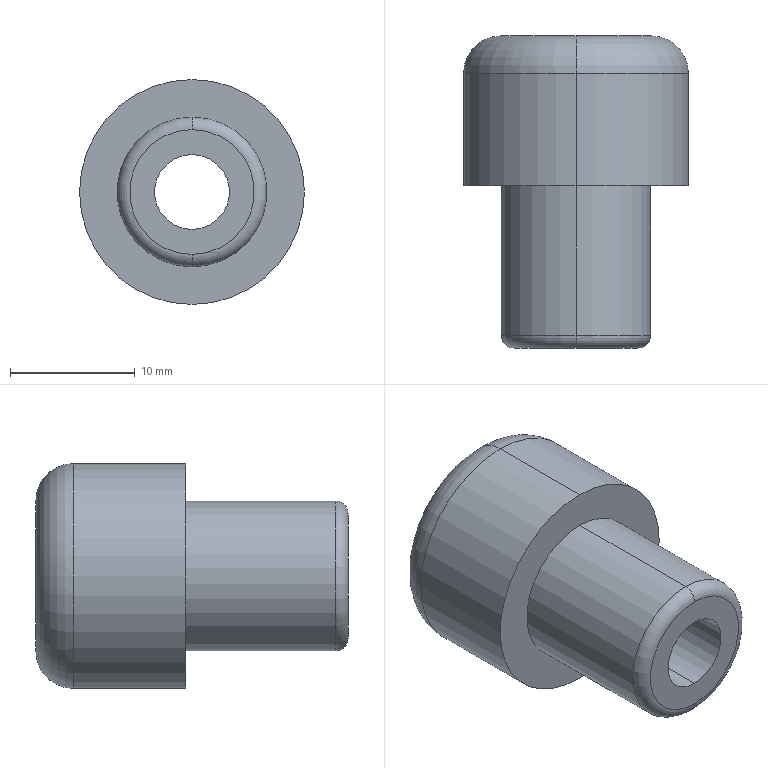Part | SolidWorks | features Fillet 2, Revolution 1 | 1 solid | 13 faces | box 18 x 25 x 18 mm | volume 3708 mm3 | cylinder 6 | torus 4 | plane 3 | commonest cylinder face diameters 6 x2 12 x2 18 x2
STEP:
#1=CARTESIAN_POINT('',(0.,1.,6.));
#2=VERTEX_POINT('',#1);
#3=CARTESIAN_POINT('',(0.,1.,-6.));
#4=VERTEX_POINT('',#3);
#5=CARTESIAN_POINT('',(0.,1.,0.));
#6=DIRECTION('',(0.,1.,0.));
#7=DIRECTION('',(0.,0.,-1.));
#8=AXIS2_PLACEMENT_3D('',#5,#6,#7);
#9=CIRCLE('',#8,6.);
#10=EDGE_CURVE('',#2,#4,#9,.T.);
#11=ORIENTED_EDGE('',*,*,#10,.F.);
#12=CARTESIAN_POINT('',(0.,0.,5.));
#13=VERTEX_POINT('',#12);
#14=CARTESIAN_POINT('',(0.,1.,5.));
#15=DIRECTION('',(1.,0.,0.));
#16=DIRECTION('',(0.,0.,-1.));
#17=AXIS2_PLACEMENT_3D('',#14,#15,#16);
#18=CIRCLE('',#17,1.);
#19=EDGE_CURVE('',#2,#13,#18,.T.);
#20=ORIENTED_EDGE('',*,*,#19,.T.);
#21=CARTESIAN_POINT('',(0.,0.,-5.));
#22=VERTEX_POINT('',#21);
#23=CARTESIAN_POINT('',(0.,0.,0.));
#24=DIRECTION('',(0.,-1.,0.));
#25=DIRECTION('',(0.,0.,-1.));
#26=AXIS2_PLACEMENT_3D('',#23,#24,#25);
#27=CIRCLE('',#26,5.);
#28=EDGE_CURVE('',#22,#13,#27,.T.);
#29=ORIENTED_EDGE('',*,*,#28,.F.);
#30=CARTESIAN_POINT('',(0.,1.,-5.));
#31=DIRECTION('',(-1.,0.,0.));
#32=DIRECTION('',(0.,0.,1.));
#33=AXIS2_PLACEMENT_3D('',#30,#31,#32);
#34=CIRCLE('',#33,1.);
#35=EDGE_CURVE('',#4,#22,#34,.T.);
#36=ORIENTED_EDGE('',*,*,#35,.F.);
#37=EDGE_LOOP('',(#11,#20,#29,#36));
#38=FACE_OUTER_BOUND('',#37,.T.);
#39=CARTESIAN_POINT('',(0.,1.,0.));
#40=DIRECTION('',(0.,-1.,0.));
#41=DIRECTION('',(0.,0.,-1.));
#42=AXIS2_PLACEMENT_3D('',#39,#40,#41);
#43=TOROIDAL_SURFACE('',#42,5.,1.);
#44=ADVANCED_FACE('',(#38),#43,.T.);
#45=CARTESIAN_POINT('',(0.,22.,-9.));
#46=VERTEX_POINT('',#45);
#47=CARTESIAN_POINT('',(0.,22.,9.));
#48=VERTEX_POINT('',#47);
#49=CARTESIAN_POINT('',(0.,22.,0.));
#50=DIRECTION('',(0.,-1.,0.));
#51=DIRECTION('',(0.,0.,1.));
#52=AXIS2_PLACEMENT_3D('',#49,#50,#51);
#53=CIRCLE('',#52,9.);
#54=EDGE_CURVE('',#46,#48,#53,.T.);
#55=ORIENTED_EDGE('',*,*,#54,.F.);
#56=CARTESIAN_POINT('',(0.,25.,-6.));
#57=VERTEX_POINT('',#56);
#58=CARTESIAN_POINT('',(0.,22.,-6.));
#59=DIRECTION('',(1.,0.,0.));
#60=DIRECTION('',(0.,0.,-1.));
#61=AXIS2_PLACEMENT_3D('',#58,#59,#60);
#62=CIRCLE('',#61,3.);
#63=EDGE_CURVE('',#46,#57,#62,.T.);
#64=ORIENTED_EDGE('',*,*,#63,.T.);
#65=CARTESIAN_POINT('',(0.,25.,6.));
#66=VERTEX_POINT('',#65);
#67=CARTESIAN_POINT('',(0.,25.,0.));
#68=DIRECTION('',(0.,1.,0.));
#69=DIRECTION('',(0.,0.,1.));
#70=AXIS2_PLACEMENT_3D('',#67,#68,#69);
#71=CIRCLE('',#70,6.);
#72=EDGE_CURVE('',#66,#57,#71,.T.);
#73=ORIENTED_EDGE('',*,*,#72,.F.);
#74=CARTESIAN_POINT('',(0.,22.,6.));
#75=DIRECTION('',(-1.,0.,0.));
#76=DIRECTION('',(0.,0.,1.));
#77=AXIS2_PLACEMENT_3D('',#74,#75,#76);
#78=CIRCLE('',#77,3.);
#79=EDGE_CURVE('',#48,#66,#78,.T.);
#80=ORIENTED_EDGE('',*,*,#79,.F.);
#81=EDGE_LOOP('',(#55,#64,#73,#80));
#82=FACE_OUTER_BOUND('',#81,.T.);
#83=CARTESIAN_POINT('',(0.,22.,0.));
#84=DIRECTION('',(0.,1.,0.));
#85=DIRECTION('',(0.,0.,1.));
#86=AXIS2_PLACEMENT_3D('',#83,#84,#85);
#87=TOROIDAL_SURFACE('',#86,6.,3.);
#88=ADVANCED_FACE('',(#82),#87,.T.);
#89=ORIENTED_EDGE('',*,*,#54,.T.);
#90=CARTESIAN_POINT('',(0.,13.,9.));
#91=VERTEX_POINT('',#90);
#92=CARTESIAN_POINT('',(0.,0.,9.));
#93=DIRECTION('',(0.,-1.,0.));
#94=VECTOR('',#93,1000.);
#95=LINE('',#92,#94);
#96=EDGE_CURVE('',#48,#91,#95,.T.);
#97=ORIENTED_EDGE('',*,*,#96,.T.);
#98=CARTESIAN_POINT('',(0.,13.,-9.));
#99=VERTEX_POINT('',#98);
#100=CARTESIAN_POINT('',(0.,13.,0.));
#101=DIRECTION('',(0.,-1.,0.));
#102=DIRECTION('',(0.,0.,-1.));
#103=AXIS2_PLACEMENT_3D('',#100,#101,#102);
#104=CIRCLE('',#103,9.);
#105=EDGE_CURVE('',#99,#91,#104,.T.);
#106=ORIENTED_EDGE('',*,*,#105,.F.);
#107=CARTESIAN_POINT('',(0.,0.,-9.));
#108=DIRECTION('',(0.,-1.,0.));
#109=VECTOR('',#108,1000.);
#110=LINE('',#107,#109);
#111=EDGE_CURVE('',#46,#99,#110,.T.);
#112=ORIENTED_EDGE('',*,*,#111,.F.);
#113=EDGE_LOOP('',(#89,#97,#106,#112));
#114=FACE_OUTER_BOUND('',#113,.T.);
#115=CARTESIAN_POINT('',(0.,0.,0.));
#116=DIRECTION('',(0.,-1.,0.));
#117=DIRECTION('',(0.,0.,-1.));
#118=AXIS2_PLACEMENT_3D('',#115,#116,#117);
#119=CYLINDRICAL_SURFACE('',#118,9.);
#120=ADVANCED_FACE('',(#114),#119,.T.);
#121=CARTESIAN_POINT('',(0.,13.,-6.));
#122=VERTEX_POINT('',#121);
#123=CARTESIAN_POINT('',(0.,13.,6.));
#124=VERTEX_POINT('',#123);
#125=CARTESIAN_POINT('',(0.,13.,0.));
#126=DIRECTION('',(0.,-1.,0.));
#127=DIRECTION('',(0.,0.,-1.));
#128=AXIS2_PLACEMENT_3D('',#125,#126,#127);
#129=CIRCLE('',#128,6.);
#130=EDGE_CURVE('',#122,#124,#129,.T.);
#131=ORIENTED_EDGE('',*,*,#130,.T.);
#132=CARTESIAN_POINT('',(0.,0.,6.));
#133=DIRECTION('',(0.,-1.,0.));
#134=VECTOR('',#133,1000.);
#135=LINE('',#132,#134);
#136=EDGE_CURVE('',#124,#2,#135,.T.);
#137=ORIENTED_EDGE('',*,*,#136,.T.);
#138=ORIENTED_EDGE('',*,*,#10,.T.);
#139=CARTESIAN_POINT('',(0.,0.,-6.));
#140=DIRECTION('',(0.,-1.,0.));
#141=VECTOR('',#140,1000.);
#142=LINE('',#139,#141);
#143=EDGE_CURVE('',#122,#4,#142,.T.);
#144=ORIENTED_EDGE('',*,*,#143,.F.);
#145=EDGE_LOOP('',(#131,#137,#138,#144));
#146=FACE_OUTER_BOUND('',#145,.T.);
#147=CARTESIAN_POINT('',(0.,0.,0.));
#148=DIRECTION('',(0.,-1.,0.));
#149=DIRECTION('',(0.,0.,-1.));
#150=AXIS2_PLACEMENT_3D('',#147,#148,#149);
#151=CYLINDRICAL_SURFACE('',#150,6.);
#152=ADVANCED_FACE('',(#146),#151,.T.);
#153=CARTESIAN_POINT('',(0.,25.,3.));
#154=VERTEX_POINT('',#153);
#155=CARTESIAN_POINT('',(0.,25.,-3.));
#156=VERTEX_POINT('',#155);
#157=CARTESIAN_POINT('',(0.,25.,0.));
#158=DIRECTION('',(0.,-1.,0.));
#159=DIRECTION('',(0.,0.,-1.));
#160=AXIS2_PLACEMENT_3D('',#157,#158,#159);
#161=CIRCLE('',#160,3.);
#162=EDGE_CURVE('',#154,#156,#161,.T.);
#163=ORIENTED_EDGE('',*,*,#162,.F.);
#164=CARTESIAN_POINT('',(0.,0.,3.));
#165=VERTEX_POINT('',#164);
#166=CARTESIAN_POINT('',(0.,0.,3.));
#167=DIRECTION('',(0.,-1.,0.));
#168=VECTOR('',#167,1000.);
#169=LINE('',#166,#168);
#170=EDGE_CURVE('',#154,#165,#169,.T.);
#171=ORIENTED_EDGE('',*,*,#170,.T.);
#172=CARTESIAN_POINT('',(0.,0.,-3.));
#173=VERTEX_POINT('',#172);
#174=CARTESIAN_POINT('',(0.,0.,0.));
#175=DIRECTION('',(0.,-1.,0.));
#176=DIRECTION('',(0.,0.,-1.));
#177=AXIS2_PLACEMENT_3D('',#174,#175,#176);
#178=CIRCLE('',#177,3.);
#179=EDGE_CURVE('',#165,#173,#178,.T.);
#180=ORIENTED_EDGE('',*,*,#179,.T.);
#181=CARTESIAN_POINT('',(0.,0.,-3.));
#182=DIRECTION('',(0.,-1.,0.));
#183=VECTOR('',#182,1000.);
#184=LINE('',#181,#183);
#185=EDGE_CURVE('',#156,#173,#184,.T.);
#186=ORIENTED_EDGE('',*,*,#185,.F.);
#187=EDGE_LOOP('',(#163,#171,#180,#186));
#188=FACE_OUTER_BOUND('',#187,.T.);
#189=CARTESIAN_POINT('',(0.,0.,0.));
#190=DIRECTION('',(0.,-1.,0.));
#191=DIRECTION('',(0.,0.,-1.));
#192=AXIS2_PLACEMENT_3D('',#189,#190,#191);
#193=CYLINDRICAL_SURFACE('',#192,3.);
#194=ADVANCED_FACE('',(#188),#193,.F.);
#195=ORIENTED_EDGE('',*,*,#72,.T.);
#196=CARTESIAN_POINT('',(0.,25.,0.));
#197=DIRECTION('',(0.,1.,0.));
#198=DIRECTION('',(0.,0.,1.));
#199=AXIS2_PLACEMENT_3D('',#196,#197,#198);
#200=CIRCLE('',#199,6.);
#201=EDGE_CURVE('',#57,#66,#200,.T.);
#202=ORIENTED_EDGE('',*,*,#201,.T.);
#203=EDGE_LOOP('',(#195,#202));
#204=FACE_OUTER_BOUND('',#203,.T.);
#205=CARTESIAN_POINT('',(0.,25.,0.));
#206=DIRECTION('',(0.,-1.,0.));
#207=DIRECTION('',(0.,0.,-1.));
#208=AXIS2_PLACEMENT_3D('',#205,#206,#207);
#209=CIRCLE('',#208,3.);
#210=EDGE_CURVE('',#156,#154,#209,.T.);
#211=ORIENTED_EDGE('',*,*,#210,.T.);
#212=ORIENTED_EDGE('',*,*,#162,.T.);
#213=EDGE_LOOP('',(#211,#212));
#214=FACE_BOUND('',#213,.T.);
#215=CARTESIAN_POINT('',(9.,25.,0.));
#216=DIRECTION('',(0.,1.,0.));
#217=DIRECTION('',(0.,0.,1.));
#218=AXIS2_PLACEMENT_3D('',#215,#216,#217);
#219=PLANE('',#218);
#220=ADVANCED_FACE('',(#204,#214),#219,.T.);
#221=ORIENTED_EDGE('',*,*,#170,.F.);
#222=ORIENTED_EDGE('',*,*,#210,.F.);
#223=ORIENTED_EDGE('',*,*,#185,.T.);
#224=CARTESIAN_POINT('',(0.,0.,0.));
#225=DIRECTION('',(0.,-1.,0.));
#226=DIRECTION('',(0.,0.,-1.));
#227=AXIS2_PLACEMENT_3D('',#224,#225,#226);
#228=CIRCLE('',#227,3.);
#229=EDGE_CURVE('',#173,#165,#228,.T.);
#230=ORIENTED_EDGE('',*,*,#229,.T.);
#231=EDGE_LOOP('',(#221,#222,#223,#230));
#232=FACE_OUTER_BOUND('',#231,.T.);
#233=CARTESIAN_POINT('',(0.,0.,0.));
#234=DIRECTION('',(0.,-1.,0.));
#235=DIRECTION('',(0.,0.,-1.));
#236=AXIS2_PLACEMENT_3D('',#233,#234,#235);
#237=CYLINDRICAL_SURFACE('',#236,3.);
#238=ADVANCED_FACE('',(#232),#237,.F.);
#239=ORIENTED_EDGE('',*,*,#28,.T.);
#240=CARTESIAN_POINT('',(0.,0.,0.));
#241=DIRECTION('',(0.,-1.,0.));
#242=DIRECTION('',(0.,0.,-1.));
#243=AXIS2_PLACEMENT_3D('',#240,#241,#242);
#244=CIRCLE('',#243,5.);
#245=EDGE_CURVE('',#13,#22,#244,.T.);
#246=ORIENTED_EDGE('',*,*,#245,.T.);
#247=EDGE_LOOP('',(#239,#246));
#248=FACE_OUTER_BOUND('',#247,.T.);
#249=ORIENTED_EDGE('',*,*,#229,.F.);
#250=ORIENTED_EDGE('',*,*,#179,.F.);
#251=EDGE_LOOP('',(#249,#250));
#252=FACE_BOUND('',#251,.T.);
#253=CARTESIAN_POINT('',(3.,0.,0.));
#254=DIRECTION('',(0.,-1.,0.));
#255=DIRECTION('',(0.,0.,-1.));
#256=AXIS2_PLACEMENT_3D('',#253,#254,#255);
#257=PLANE('',#256);
#258=ADVANCED_FACE('',(#248,#252),#257,.T.);
#259=ORIENTED_EDGE('',*,*,#136,.F.);
#260=CARTESIAN_POINT('',(0.,13.,0.));
#261=DIRECTION('',(0.,-1.,0.));
#262=DIRECTION('',(0.,0.,-1.));
#263=AXIS2_PLACEMENT_3D('',#260,#261,#262);
#264=CIRCLE('',#263,6.);
#265=EDGE_CURVE('',#124,#122,#264,.T.);
#266=ORIENTED_EDGE('',*,*,#265,.T.);
#267=ORIENTED_EDGE('',*,*,#143,.T.);
#268=CARTESIAN_POINT('',(0.,1.,0.));
#269=DIRECTION('',(0.,1.,0.));
#270=DIRECTION('',(0.,0.,-1.));
#271=AXIS2_PLACEMENT_3D('',#268,#269,#270);
#272=CIRCLE('',#271,6.);
#273=EDGE_CURVE('',#4,#2,#272,.T.);
#274=ORIENTED_EDGE('',*,*,#273,.T.);
#275=EDGE_LOOP('',(#259,#266,#267,#274));
#276=FACE_OUTER_BOUND('',#275,.T.);
#277=CARTESIAN_POINT('',(0.,0.,0.));
#278=DIRECTION('',(0.,-1.,0.));
#279=DIRECTION('',(0.,0.,-1.));
#280=AXIS2_PLACEMENT_3D('',#277,#278,#279);
#281=CYLINDRICAL_SURFACE('',#280,6.);
#282=ADVANCED_FACE('',(#276),#281,.T.);
#283=ORIENTED_EDGE('',*,*,#105,.T.);
#284=CARTESIAN_POINT('',(0.,13.,0.));
#285=DIRECTION('',(0.,-1.,0.));
#286=DIRECTION('',(0.,0.,-1.));
#287=AXIS2_PLACEMENT_3D('',#284,#285,#286);
#288=CIRCLE('',#287,9.);
#289=EDGE_CURVE('',#91,#99,#288,.T.);
#290=ORIENTED_EDGE('',*,*,#289,.T.);
#291=EDGE_LOOP('',(#283,#290));
#292=FACE_OUTER_BOUND('',#291,.T.);
#293=ORIENTED_EDGE('',*,*,#130,.F.);
#294=ORIENTED_EDGE('',*,*,#265,.F.);
#295=EDGE_LOOP('',(#293,#294));
#296=FACE_BOUND('',#295,.T.);
#297=CARTESIAN_POINT('',(6.,13.,0.));
#298=DIRECTION('',(0.,-1.,0.));
#299=DIRECTION('',(0.,0.,-1.));
#300=AXIS2_PLACEMENT_3D('',#297,#298,#299);
#301=PLANE('',#300);
#302=ADVANCED_FACE('',(#292,#296),#301,.T.);
#303=ORIENTED_EDGE('',*,*,#96,.F.);
#304=CARTESIAN_POINT('',(0.,22.,0.));
#305=DIRECTION('',(0.,-1.,0.));
#306=DIRECTION('',(0.,0.,1.));
#307=AXIS2_PLACEMENT_3D('',#304,#305,#306);
#308=CIRCLE('',#307,9.);
#309=EDGE_CURVE('',#48,#46,#308,.T.);
#310=ORIENTED_EDGE('',*,*,#309,.T.);
#311=ORIENTED_EDGE('',*,*,#111,.T.);
#312=ORIENTED_EDGE('',*,*,#289,.F.);
#313=EDGE_LOOP('',(#303,#310,#311,#312));
#314=FACE_OUTER_BOUND('',#313,.T.);
#315=CARTESIAN_POINT('',(0.,0.,0.));
#316=DIRECTION('',(0.,-1.,0.));
#317=DIRECTION('',(0.,0.,-1.));
#318=AXIS2_PLACEMENT_3D('',#315,#316,#317);
#319=CYLINDRICAL_SURFACE('',#318,9.);
#320=ADVANCED_FACE('',(#314),#319,.T.);
#321=ORIENTED_EDGE('',*,*,#63,.F.);
#322=ORIENTED_EDGE('',*,*,#309,.F.);
#323=ORIENTED_EDGE('',*,*,#79,.T.);
#324=ORIENTED_EDGE('',*,*,#201,.F.);
#325=EDGE_LOOP('',(#321,#322,#323,#324));
#326=FACE_OUTER_BOUND('',#325,.T.);
#327=CARTESIAN_POINT('',(0.,22.,0.));
#328=DIRECTION('',(0.,1.,0.));
#329=DIRECTION('',(0.,0.,1.));
#330=AXIS2_PLACEMENT_3D('',#327,#328,#329);
#331=TOROIDAL_SURFACE('',#330,6.,3.);
#332=ADVANCED_FACE('',(#326),#331,.T.);
#333=ORIENTED_EDGE('',*,*,#19,.F.);
#334=ORIENTED_EDGE('',*,*,#273,.F.);
#335=ORIENTED_EDGE('',*,*,#35,.T.);
#336=ORIENTED_EDGE('',*,*,#245,.F.);
#337=EDGE_LOOP('',(#333,#334,#335,#336));
#338=FACE_OUTER_BOUND('',#337,.T.);
#339=CARTESIAN_POINT('',(0.,1.,0.));
#340=DIRECTION('',(0.,-1.,0.));
#341=DIRECTION('',(0.,0.,-1.));
#342=AXIS2_PLACEMENT_3D('',#339,#340,#341);
#343=TOROIDAL_SURFACE('',#342,5.,1.);
#344=ADVANCED_FACE('',(#338),#343,.T.);
#345=CLOSED_SHELL('',(#44,#88,#120,#152,#194,#220,#238,#258,#282,#302,#320,#332,#344));
#346=MANIFOLD_SOLID_BREP('',#345);
#347=CARTESIAN_POINT('',(0.,0.,0.));
#348=DIRECTION('',(0.,0.,1.));
#349=DIRECTION('',(1.,0.,0.));
#350=AXIS2_PLACEMENT_3D('',#347,#348,#349);
#351=(LENGTH_UNIT()NAMED_UNIT(*)SI_UNIT(.MILLI.,.METRE.));
#352=UNCERTAINTY_MEASURE_WITH_UNIT(LENGTH_MEASURE(0.00001),#351,'','');
#353=(NAMED_UNIT(*)PLANE_ANGLE_UNIT()SI_UNIT($,.RADIAN.));
#354=(NAMED_UNIT(*)SI_UNIT($,.STERADIAN.)SOLID_ANGLE_UNIT());
#355=(GEOMETRIC_REPRESENTATION_CONTEXT(3)GLOBAL_UNCERTAINTY_ASSIGNED_CONTEXT((#352))GLOBAL_UNIT_ASSIGNED_CONTEXT((#351,#353,#354))REPRESENTATION_CONTEXT('',''));
#356=ADVANCED_BREP_SHAPE_REPRESENTATION('',(#346,#350),#355);